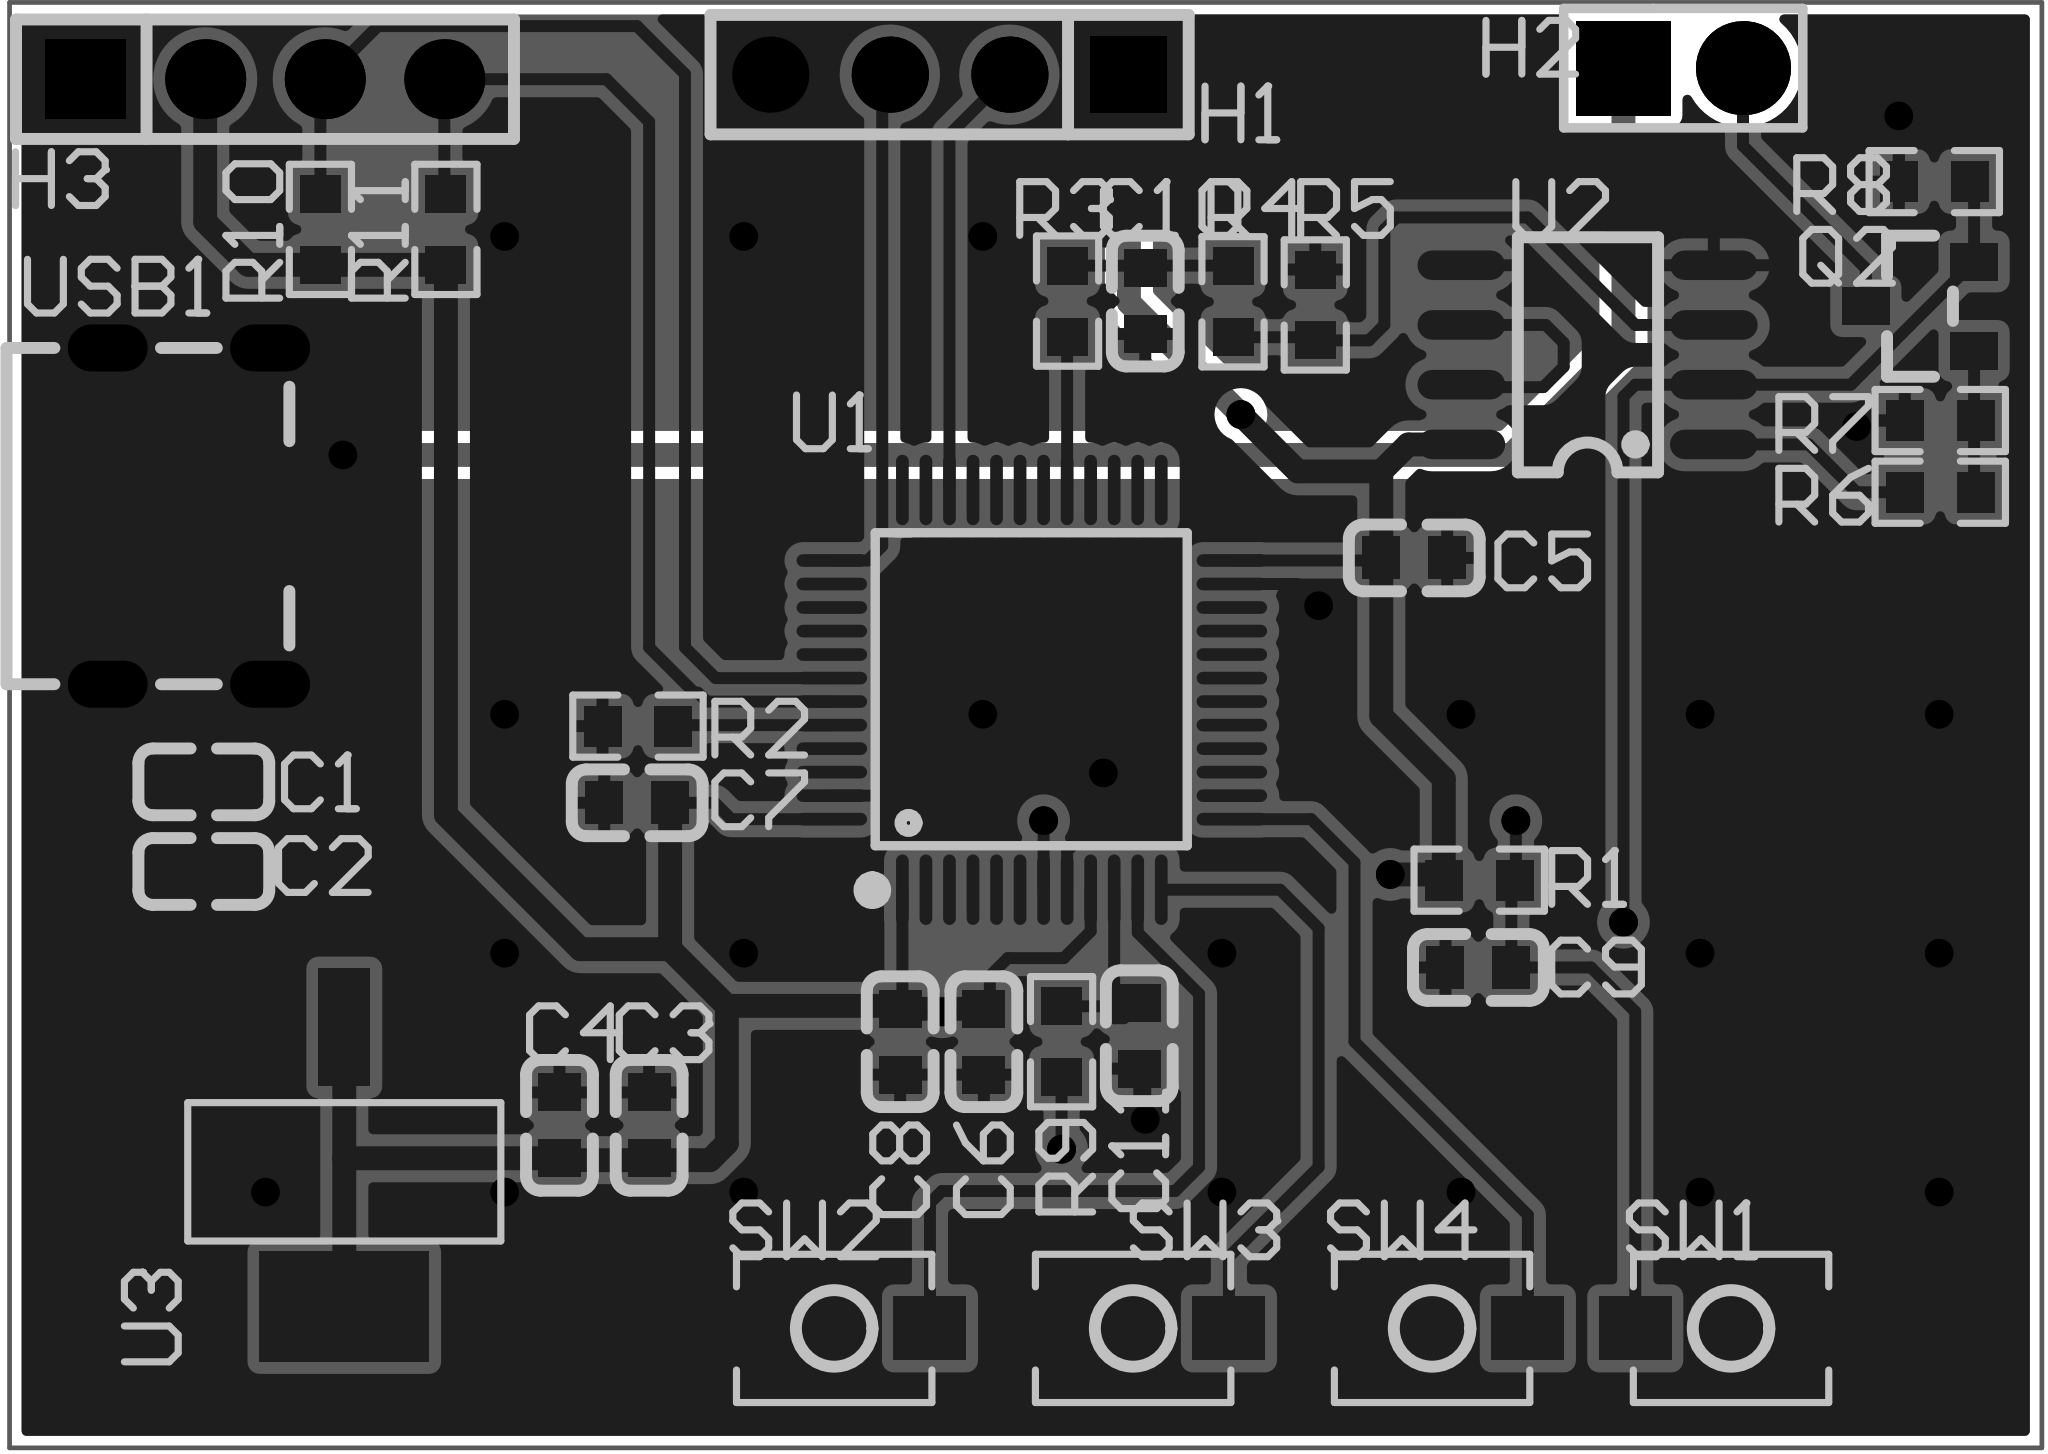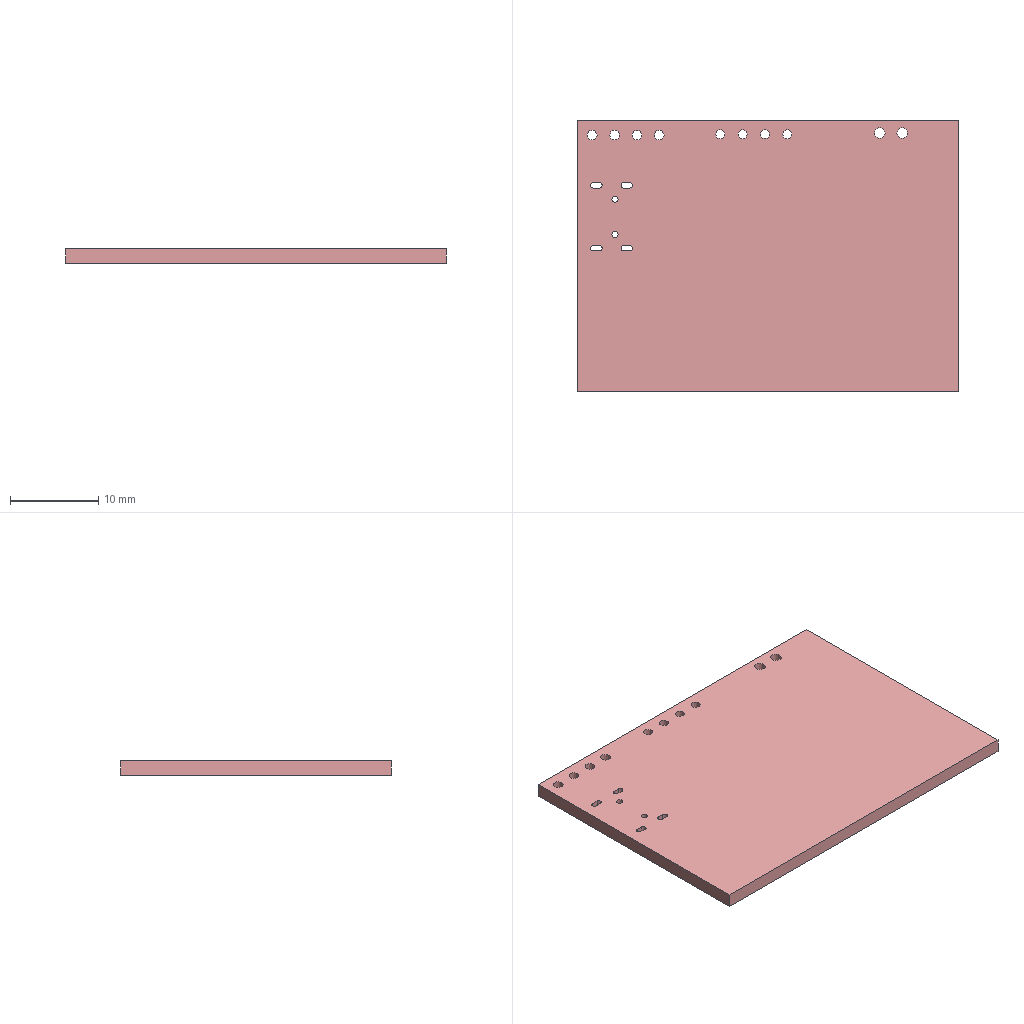Circuit board layout | Altium Designer | box 43.2 x 30.7 x 1.6 mm
Layer stack:
# Altium Designer layer stack of  (unit mm; dielectric type: 0 none, 1 core, 2 prepreg, 3 surface material)
index,name,kind,layer,copper_thickness_mm,dielectric_type,dielectric_thickness_mm,dielectric_material,dielectric_constant
0,Top Paste Mask Layer,other,,,,,,
1,Top Silkscreen Layer,other,,,,,,
2,Top Solder Mask Layer,dielectric,,,3,0.01,,3.3
3,Top Layer,copper,Top Layer,0.035,,,,
4,Dielectric1,dielectric,,,3,1.51,FR4,4.5
5,Bottom Layer,copper,Bottom Layer,0.035,,,,
6,Bottom Solder Mask Layer,dielectric,,,3,0.01,,3.3
7,Bottom Silkscreen Layer,other,,,,,,
8,Bottom Paste Mask Layer,other,,,,,,
# drill layer pairs: low layer,high layer
drill_pair,Top Layer,Bottom Layer
Part placement:
Designator,Comment,Layer,Footprint,Center-X(mm),Center-Y(mm),Rotation
C1,10uf,TopLayer,C0603,81.978,92.011,0
C2,0.1uf,TopLayer,C0603,81.978,90.106,0
C3,10uf,TopLayer,C0603,91.44,84.709,270
C4,0.1uf,TopLayer,C0603,89.535,84.709,270
C5,0.1uf,TopLayer,C0603,107.696,96.774,180
C6,0.1uf,TopLayer,C0603,98.552,86.487,90
C7,0.1uf,TopLayer,C0603,91.186,91.567,0
C8,0.1uf,TopLayer,C0603,96.774,86.487,90
C9,0.1uf,TopLayer,C0603,109.059,88.066,0
C10,1uf,TopLayer,C0603,101.981,102.235,270
C11,100nF,TopLayer,C0603,101.854,86.614,90
H1,HX PH254-01-04-Z-L11.5 straight pin header,TopLayer,HDR-TH_4P-HX-PH254-01-04-Z-L11.5,97.824,107.05,180
H2,HX PH254-01-02-Z-L11.5 male header connector,TopLayer,HDR-TH_2P-P2.54-V-M,113.411,107.188,0
H3,2.54-1*4P female,TopLayer,HDR-TH_4P-P2.54-V-F,83.278,106.952,0
Q2,AO3400,TopLayer,SOT-23_L2.9-W1.3-P1.90-LS2.4-BR,118.441,102.126,0
R1,10K,TopLayer,R0603,109.076,89.923,180
R2,100K,TopLayer,R0603,91.203,93.198,180
R3,10K,TopLayer,R0603,100.33,102.235,90
R4,3.3k,TopLayer,R0603,103.845,102.22,270
R5,5.1k,TopLayer,R0603,105.593,102.152,90
R6,100,TopLayer,R0603,118.872,98.171,0
R7,100K,TopLayer,R0603,118.872,99.695,0
R8,10K,TopLayer,R0603,118.745,104.775,0
R9,10K,TopLayer,R0603,100.203,86.487,90
R10,4.7K,TopLayer,R0603,84.455,103.759,90
R11,4.7K,TopLayer,R0603,87.122,103.759,90
SW1,,TopLayer,Key_SMD_3x4x2,114.427,80.391,0
SW2,,TopLayer,Key_SMD_3x4x2,95.372,80.391,180
SW3,,TopLayer,Key_SMD_3x4x2,101.724,80.391,180
SW4,,TopLayer,Key_SMD_3x4x2,108.075,80.391,180
U1,AT32F421C8T7,TopLayer,LQFP-48_L7.0-W7.0-P0.50-LS9.0-BL,99.571,93.969,0
U2,LMV358,TopLayer,SOP-8_L4.9-W3.9-P1.27-LS6.0-BL,111.379,101.092,90
U3,AMS1117-3.3(XBLW),TopLayer,SOT-223-3_L6.5-W3.4-P2.30-LS7.0-BR-1,84.963,83.82,90
USB1,,TopLayer,USB_Micro,81.661,97.663,270
Pad and via stacks:
# Altium Designer via and pad stacks of  (unit mm). Each distinct definition once, with the count of objects using it.
# via: kind,start_layer,end_layer,hole_mm,diameter_mm,mode(0 simple;1 top-mid-bottom;2 full stack),diameter_per_layer,count,example_net
# pad: kind,layer,hole_mm,hole_type(0 round;1 square;2 slot),plating,top_size,top_shape(1 round;2 rect;3 octagon;9 rounded rect),mid_size,bottom_size,mode,footprint,size_per_layer,count,example
pad,Top Layer,0,0,plated,0.8x0.9,2,0.8x0.9,0.8x0.9,0,C0603,,22,C1.2
pad,Top Layer,0,0,plated,1x0.8,2,1x0.8,1x0.8,0,SOT-23_L2.9-W1.3-P1.90-LS2.4-BR,,3,Q2.2
pad,Top Layer,0,0,plated,0.8065x0.864,2,0.8065x0.864,0.8065x0.864,0,R0603,,22,R1.2
pad,Top Layer,0,0,plated,1.53x1.36,2,1.53x1.36,1.53x1.36,0,Key_SMD_3x4x2,,8,SW1.1
pad,Top Layer,0,0,plated,0.27x1.5,1,0.27x1.5,0.27x1.5,0,LQFP-48_L7.0-W7.0-P0.50-LS9.0-BL,,24,U1.1
pad,Top Layer,0,0,plated,1.5x0.27,1,1.5x0.27,1.5x0.27,0,LQFP-48_L7.0-W7.0-P0.50-LS9.0-BL,,24,U1.13
pad,Top Layer,0,0,plated,0.63x1.865,1,0.63x1.865,0.63x1.865,0,SOP-8_L4.9-W3.9-P1.27-LS6.0-BL,,8,U2.1
pad,Top Layer,0,0,plated,2.34x3.6,2,2.34x3.6,2.34x3.6,0,SOT-223-3_L6.5-W3.4-P2.30-LS7.0-BR-1,,1,U3.2
pad,Top Layer,0,0,plated,2.5x1.1,2,2.5x1.1,2.5x1.1,0,SOT-223-3_L6.5-W3.4-P2.30-LS7.0-BR-1,,3,U3.3
pad,Top Layer,0,0,plated,0.4x1.4,2,0.4x1.4,0.4x1.4,0,USB_Micro,,5,USB1.1
pad,Multi-Layer,1.02,0,plated,1.62x1.62,1,1.62x1.62,1.62x1.62,0,HDR-TH_4P-HX-PH254-01-04-Z-L11.5,,3,H1.4
pad,Multi-Layer,1.02,0,plated,1.62x1.62,2,1.62x1.62,1.62x1.62,0,HDR-TH_4P-HX-PH254-01-04-Z-L11.5,,1,H1.1
pad,Multi-Layer,1.2,0,plated,2x2,2,2x2,2x2,0,HDR-TH_2P-P2.54-V-M,,1,H2.1
pad,Multi-Layer,1.2,0,plated,2x2,1,2x2,2x2,0,HDR-TH_2P-P2.54-V-M,,1,H2.2
pad,Multi-Layer,1.1,0,plated,1.7x1.7,2,1.7x1.7,1.7x1.7,0,HDR-TH_4P-P2.54-V-F,,1,H3.1
pad,Multi-Layer,1.1,0,plated,1.7x1.7,1,1.7x1.7,1.7x1.7,0,HDR-TH_4P-P2.54-V-F,,3,H3.2
pad,Multi-Layer,0.6,2,plated,1x1.7,1,1x1.7,1x1.7,0,USB_Micro,,4,USB1.6
via,Top Layer,Bottom Layer,0.3048,0.61,0,,33,NRES
Copper pours:
name,layer,net,type(0 solid;1 hatched;2 none)
Top Layer-GND,Top Layer,GND,0
Bottom Layer-GND,Bottom Layer,GND,0